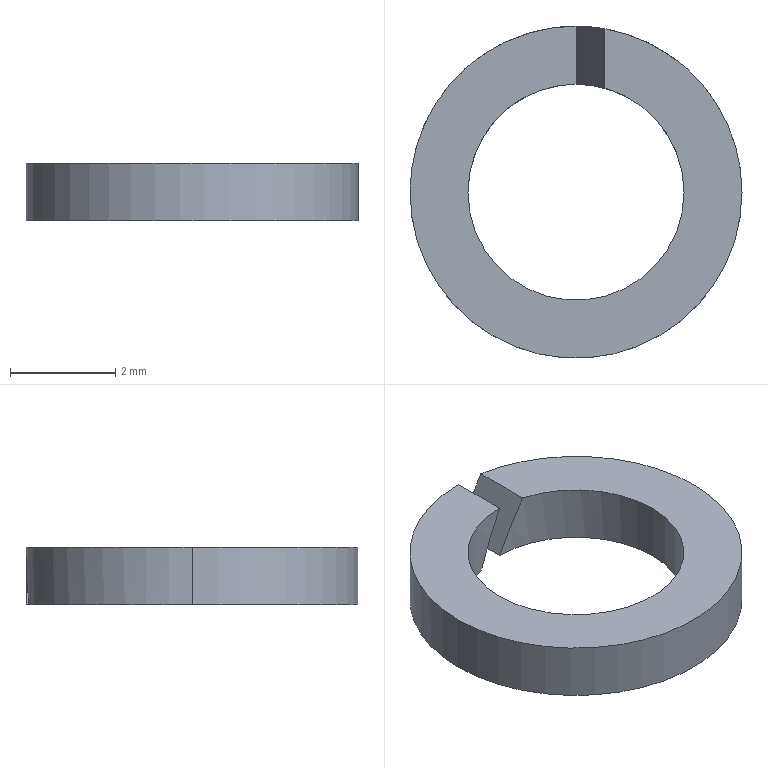Part | STEP file | Guide wheel mechanism revised.sldasm-Part-510 | 1 solid | 10 faces | box 6.3 x 6.3 x 1.1 mm | volume 19.099 mm3 | cylinder 6 | plane 4 | commonest cylinder face diameters 4.1 x3 6.3 x3
STEP:
#1=CARTESIAN_POINT('',(2.05,0.,0.));
#2=VERTEX_POINT('',#1);
#3=CARTESIAN_POINT('',(-2.05,0.,0.));
#4=VERTEX_POINT('',#3);
#5=CARTESIAN_POINT('',(0.,0.,0.));
#6=DIRECTION('',(0.,0.,-1.));
#7=DIRECTION('',(1.,0.,0.));
#8=AXIS2_PLACEMENT_3D('',#5,#6,#7);
#9=CIRCLE('',#8,2.05);
#10=EDGE_CURVE('',#2,#4,#9,.T.);
#11=ORIENTED_EDGE('',*,*,#10,.T.);
#12=CARTESIAN_POINT('',(-2.05,0.,1.1));
#13=VERTEX_POINT('',#12);
#14=CARTESIAN_POINT('',(-2.05,0.,0.));
#15=DIRECTION('',(0.,0.,1.));
#16=VECTOR('',#15,1000.);
#17=LINE('',#14,#16);
#18=EDGE_CURVE('',#4,#13,#17,.T.);
#19=ORIENTED_EDGE('',*,*,#18,.T.);
#20=CARTESIAN_POINT('',(2.05,0.,1.1));
#21=VERTEX_POINT('',#20);
#22=CARTESIAN_POINT('',(0.,0.,1.1));
#23=DIRECTION('',(0.,0.,-1.));
#24=DIRECTION('',(1.,0.,0.));
#25=AXIS2_PLACEMENT_3D('',#22,#23,#24);
#26=CIRCLE('',#25,2.05);
#27=EDGE_CURVE('',#21,#13,#26,.T.);
#28=ORIENTED_EDGE('',*,*,#27,.F.);
#29=CARTESIAN_POINT('',(2.05,0.,0.));
#30=DIRECTION('',(0.,0.,1.));
#31=VECTOR('',#30,1000.);
#32=LINE('',#29,#31);
#33=EDGE_CURVE('',#2,#21,#32,.T.);
#34=ORIENTED_EDGE('',*,*,#33,.F.);
#35=EDGE_LOOP('',(#11,#19,#28,#34));
#36=FACE_OUTER_BOUND('',#35,.T.);
#37=CARTESIAN_POINT('',(0.,0.,0.));
#38=DIRECTION('',(0.,0.,1.));
#39=DIRECTION('',(1.,0.,0.));
#40=AXIS2_PLACEMENT_3D('',#37,#38,#39);
#41=CYLINDRICAL_SURFACE('',#40,2.05);
#42=ADVANCED_FACE('',(#36),#41,.F.);
#43=CARTESIAN_POINT('',(0.,2.05,0.));
#44=VERTEX_POINT('',#43);
#45=CARTESIAN_POINT('',(0.,0.,0.));
#46=DIRECTION('',(0.,0.,-1.));
#47=DIRECTION('',(1.,0.,0.));
#48=AXIS2_PLACEMENT_3D('',#45,#46,#47);
#49=CIRCLE('',#48,2.05);
#50=EDGE_CURVE('',#44,#2,#49,.T.);
#51=ORIENTED_EDGE('',*,*,#50,.T.);
#52=ORIENTED_EDGE('',*,*,#33,.T.);
#53=CARTESIAN_POINT('',(0.55,1.975,1.1));
#54=VERTEX_POINT('',#53);
#55=CARTESIAN_POINT('',(0.,0.,1.1));
#56=DIRECTION('',(0.,0.,-1.));
#57=DIRECTION('',(1.,0.,0.));
#58=AXIS2_PLACEMENT_3D('',#55,#56,#57);
#59=CIRCLE('',#58,2.05);
#60=EDGE_CURVE('',#54,#21,#59,.T.);
#61=ORIENTED_EDGE('',*,*,#60,.F.);
#62=CARTESIAN_POINT('',(0.,2.05,0.));
#63=CARTESIAN_POINT('',(0.1862,2.05,0.3724));
#64=CARTESIAN_POINT('',(0.3706,2.025,0.7413));
#65=CARTESIAN_POINT('',(0.55,1.975,1.1));
#66=(BOUNDED_CURVE()B_SPLINE_CURVE(3,(#62,#63,#64,#65),.UNSPECIFIED.,.F.,.F.)B_SPLINE_CURVE_WITH_KNOTS((4,4),(4.712,4.984),.UNSPECIFIED.)CURVE()GEOMETRIC_REPRESENTATION_ITEM()RATIONAL_B_SPLINE_CURVE((1.,0.9939,0.9939,1.))REPRESENTATION_ITEM(''));
#67=EDGE_CURVE('',#44,#54,#66,.T.);
#68=ORIENTED_EDGE('',*,*,#67,.F.);
#69=EDGE_LOOP('',(#51,#52,#61,#68));
#70=FACE_OUTER_BOUND('',#69,.T.);
#71=CARTESIAN_POINT('',(0.,0.,0.));
#72=DIRECTION('',(0.,0.,1.));
#73=DIRECTION('',(1.,0.,0.));
#74=AXIS2_PLACEMENT_3D('',#71,#72,#73);
#75=CYLINDRICAL_SURFACE('',#74,2.05);
#76=ADVANCED_FACE('',(#70),#75,.F.);
#77=CARTESIAN_POINT('',(-0.55,3.102,0.));
#78=VERTEX_POINT('',#77);
#79=CARTESIAN_POINT('',(-3.15,0.,0.));
#80=VERTEX_POINT('',#79);
#81=CARTESIAN_POINT('',(0.,0.,0.));
#82=DIRECTION('',(0.,0.,1.));
#83=DIRECTION('',(1.,0.,0.));
#84=AXIS2_PLACEMENT_3D('',#81,#82,#83);
#85=CIRCLE('',#84,3.15);
#86=EDGE_CURVE('',#78,#80,#85,.T.);
#87=ORIENTED_EDGE('',*,*,#86,.T.);
#88=CARTESIAN_POINT('',(-3.15,0.,1.1));
#89=VERTEX_POINT('',#88);
#90=CARTESIAN_POINT('',(-3.15,0.,0.));
#91=DIRECTION('',(0.,0.,1.));
#92=VECTOR('',#91,1000.);
#93=LINE('',#90,#92);
#94=EDGE_CURVE('',#80,#89,#93,.T.);
#95=ORIENTED_EDGE('',*,*,#94,.T.);
#96=CARTESIAN_POINT('',(0.,3.15,1.1));
#97=VERTEX_POINT('',#96);
#98=CARTESIAN_POINT('',(0.,0.,1.1));
#99=DIRECTION('',(0.,0.,-1.));
#100=DIRECTION('',(1.,0.,0.));
#101=AXIS2_PLACEMENT_3D('',#98,#99,#100);
#102=CIRCLE('',#101,3.15);
#103=EDGE_CURVE('',#89,#97,#102,.T.);
#104=ORIENTED_EDGE('',*,*,#103,.T.);
#105=CARTESIAN_POINT('',(0.,3.15,1.1));
#106=CARTESIAN_POINT('',(-0.1845,3.15,0.731));
#107=CARTESIAN_POINT('',(-0.3683,3.134,0.3634));
#108=CARTESIAN_POINT('',(-0.55,3.102,0.));
#109=(BOUNDED_CURVE()B_SPLINE_CURVE(3,(#105,#106,#107,#108),.UNSPECIFIED.,.F.,.F.)B_SPLINE_CURVE_WITH_KNOTS((4,4),(1.571,1.746),.UNSPECIFIED.)CURVE()GEOMETRIC_REPRESENTATION_ITEM()RATIONAL_B_SPLINE_CURVE((1.,0.9974,0.9974,1.))REPRESENTATION_ITEM(''));
#110=EDGE_CURVE('',#97,#78,#109,.T.);
#111=ORIENTED_EDGE('',*,*,#110,.T.);
#112=EDGE_LOOP('',(#87,#95,#104,#111));
#113=FACE_OUTER_BOUND('',#112,.T.);
#114=CARTESIAN_POINT('',(0.,0.,0.));
#115=DIRECTION('',(0.,0.,1.));
#116=DIRECTION('',(1.,0.,0.));
#117=AXIS2_PLACEMENT_3D('',#114,#115,#116);
#118=CYLINDRICAL_SURFACE('',#117,3.15);
#119=ADVANCED_FACE('',(#113),#118,.T.);
#120=ORIENTED_EDGE('',*,*,#94,.F.);
#121=CARTESIAN_POINT('',(3.15,0.,0.));
#122=VERTEX_POINT('',#121);
#123=CARTESIAN_POINT('',(0.,0.,0.));
#124=DIRECTION('',(0.,0.,1.));
#125=DIRECTION('',(1.,0.,0.));
#126=AXIS2_PLACEMENT_3D('',#123,#124,#125);
#127=CIRCLE('',#126,3.15);
#128=EDGE_CURVE('',#80,#122,#127,.T.);
#129=ORIENTED_EDGE('',*,*,#128,.T.);
#130=CARTESIAN_POINT('',(3.15,0.,1.1));
#131=VERTEX_POINT('',#130);
#132=CARTESIAN_POINT('',(3.15,0.,0.));
#133=DIRECTION('',(0.,0.,1.));
#134=VECTOR('',#133,1000.);
#135=LINE('',#132,#134);
#136=EDGE_CURVE('',#122,#131,#135,.T.);
#137=ORIENTED_EDGE('',*,*,#136,.T.);
#138=CARTESIAN_POINT('',(0.,0.,1.1));
#139=DIRECTION('',(0.,0.,-1.));
#140=DIRECTION('',(1.,0.,0.));
#141=AXIS2_PLACEMENT_3D('',#138,#139,#140);
#142=CIRCLE('',#141,3.15);
#143=EDGE_CURVE('',#131,#89,#142,.T.);
#144=ORIENTED_EDGE('',*,*,#143,.T.);
#145=EDGE_LOOP('',(#120,#129,#137,#144));
#146=FACE_OUTER_BOUND('',#145,.T.);
#147=CARTESIAN_POINT('',(0.,0.,0.));
#148=DIRECTION('',(0.,0.,1.));
#149=DIRECTION('',(1.,0.,0.));
#150=AXIS2_PLACEMENT_3D('',#147,#148,#149);
#151=CYLINDRICAL_SURFACE('',#150,3.15);
#152=ADVANCED_FACE('',(#146),#151,.T.);
#153=ORIENTED_EDGE('',*,*,#50,.F.);
#154=CARTESIAN_POINT('',(0.,3.15,0.));
#155=VERTEX_POINT('',#154);
#156=CARTESIAN_POINT('',(0.,0.,0.));
#157=DIRECTION('',(0.,-1.,0.));
#158=VECTOR('',#157,1000.);
#159=LINE('',#156,#158);
#160=EDGE_CURVE('',#155,#44,#159,.T.);
#161=ORIENTED_EDGE('',*,*,#160,.F.);
#162=CARTESIAN_POINT('',(0.,0.,0.));
#163=DIRECTION('',(0.,0.,1.));
#164=DIRECTION('',(1.,0.,0.));
#165=AXIS2_PLACEMENT_3D('',#162,#163,#164);
#166=CIRCLE('',#165,3.15);
#167=EDGE_CURVE('',#122,#155,#166,.T.);
#168=ORIENTED_EDGE('',*,*,#167,.F.);
#169=ORIENTED_EDGE('',*,*,#128,.F.);
#170=ORIENTED_EDGE('',*,*,#86,.F.);
#171=CARTESIAN_POINT('',(-0.55,1.975,0.));
#172=VERTEX_POINT('',#171);
#173=CARTESIAN_POINT('',(-0.55,0.,0.));
#174=DIRECTION('',(0.,1.,0.));
#175=VECTOR('',#174,1000.);
#176=LINE('',#173,#175);
#177=EDGE_CURVE('',#172,#78,#176,.T.);
#178=ORIENTED_EDGE('',*,*,#177,.F.);
#179=CARTESIAN_POINT('',(0.,0.,0.));
#180=DIRECTION('',(0.,0.,-1.));
#181=DIRECTION('',(1.,0.,0.));
#182=AXIS2_PLACEMENT_3D('',#179,#180,#181);
#183=CIRCLE('',#182,2.05);
#184=EDGE_CURVE('',#4,#172,#183,.T.);
#185=ORIENTED_EDGE('',*,*,#184,.F.);
#186=ORIENTED_EDGE('',*,*,#10,.F.);
#187=EDGE_LOOP('',(#153,#161,#168,#169,#170,#178,#185,#186));
#188=FACE_OUTER_BOUND('',#187,.T.);
#189=CARTESIAN_POINT('',(0.,0.,0.));
#190=DIRECTION('',(0.,0.,1.));
#191=DIRECTION('',(1.,0.,0.));
#192=AXIS2_PLACEMENT_3D('',#189,#190,#191);
#193=PLANE('',#192);
#194=ADVANCED_FACE('',(#188),#193,.F.);
#195=ORIENTED_EDGE('',*,*,#18,.F.);
#196=ORIENTED_EDGE('',*,*,#184,.T.);
#197=CARTESIAN_POINT('',(0.,2.05,1.1));
#198=VERTEX_POINT('',#197);
#199=CARTESIAN_POINT('',(0.,2.05,1.1));
#200=CARTESIAN_POINT('',(-0.1862,2.05,0.7276));
#201=CARTESIAN_POINT('',(-0.3706,2.025,0.3587));
#202=CARTESIAN_POINT('',(-0.55,1.975,0.));
#203=(BOUNDED_CURVE()B_SPLINE_CURVE(3,(#199,#200,#201,#202),.UNSPECIFIED.,.F.,.F.)B_SPLINE_CURVE_WITH_KNOTS((4,4),(1.571,1.842),.UNSPECIFIED.)CURVE()GEOMETRIC_REPRESENTATION_ITEM()RATIONAL_B_SPLINE_CURVE((1.,0.9939,0.9939,1.))REPRESENTATION_ITEM(''));
#204=EDGE_CURVE('',#198,#172,#203,.T.);
#205=ORIENTED_EDGE('',*,*,#204,.F.);
#206=CARTESIAN_POINT('',(0.,0.,1.1));
#207=DIRECTION('',(0.,0.,-1.));
#208=DIRECTION('',(1.,0.,0.));
#209=AXIS2_PLACEMENT_3D('',#206,#207,#208);
#210=CIRCLE('',#209,2.05);
#211=EDGE_CURVE('',#13,#198,#210,.T.);
#212=ORIENTED_EDGE('',*,*,#211,.F.);
#213=EDGE_LOOP('',(#195,#196,#205,#212));
#214=FACE_OUTER_BOUND('',#213,.T.);
#215=CARTESIAN_POINT('',(0.,0.,0.));
#216=DIRECTION('',(0.,0.,1.));
#217=DIRECTION('',(1.,0.,0.));
#218=AXIS2_PLACEMENT_3D('',#215,#216,#217);
#219=CYLINDRICAL_SURFACE('',#218,2.05);
#220=ADVANCED_FACE('',(#214),#219,.F.);
#221=ORIENTED_EDGE('',*,*,#67,.T.);
#222=CARTESIAN_POINT('',(0.55,3.102,1.1));
#223=VERTEX_POINT('',#222);
#224=CARTESIAN_POINT('',(0.55,0.,1.1));
#225=DIRECTION('',(0.,-1.,0.));
#226=VECTOR('',#225,1000.);
#227=LINE('',#224,#226);
#228=EDGE_CURVE('',#223,#54,#227,.T.);
#229=ORIENTED_EDGE('',*,*,#228,.F.);
#230=CARTESIAN_POINT('',(0.,3.15,0.));
#231=CARTESIAN_POINT('',(0.1845,3.15,0.369));
#232=CARTESIAN_POINT('',(0.3683,3.134,0.7366));
#233=CARTESIAN_POINT('',(0.55,3.102,1.1));
#234=(BOUNDED_CURVE()B_SPLINE_CURVE(3,(#230,#231,#232,#233),.UNSPECIFIED.,.F.,.F.)B_SPLINE_CURVE_WITH_KNOTS((4,4),(4.712,4.888),.UNSPECIFIED.)CURVE()GEOMETRIC_REPRESENTATION_ITEM()RATIONAL_B_SPLINE_CURVE((1.,0.9974,0.9974,1.))REPRESENTATION_ITEM(''));
#235=EDGE_CURVE('',#155,#223,#234,.T.);
#236=ORIENTED_EDGE('',*,*,#235,.F.);
#237=ORIENTED_EDGE('',*,*,#160,.T.);
#238=EDGE_LOOP('',(#221,#229,#236,#237));
#239=FACE_OUTER_BOUND('',#238,.T.);
#240=CARTESIAN_POINT('',(0.55,0.,1.1));
#241=DIRECTION('',(0.8944,0.,-0.4472));
#242=DIRECTION('',(-0.4472,0.,-0.8944));
#243=AXIS2_PLACEMENT_3D('',#240,#241,#242);
#244=PLANE('',#243);
#245=ADVANCED_FACE('',(#239),#244,.F.);
#246=ORIENTED_EDGE('',*,*,#136,.F.);
#247=ORIENTED_EDGE('',*,*,#167,.T.);
#248=ORIENTED_EDGE('',*,*,#235,.T.);
#249=CARTESIAN_POINT('',(0.,0.,1.1));
#250=DIRECTION('',(0.,0.,-1.));
#251=DIRECTION('',(1.,0.,0.));
#252=AXIS2_PLACEMENT_3D('',#249,#250,#251);
#253=CIRCLE('',#252,3.15);
#254=EDGE_CURVE('',#223,#131,#253,.T.);
#255=ORIENTED_EDGE('',*,*,#254,.T.);
#256=EDGE_LOOP('',(#246,#247,#248,#255));
#257=FACE_OUTER_BOUND('',#256,.T.);
#258=CARTESIAN_POINT('',(0.,0.,0.));
#259=DIRECTION('',(0.,0.,1.));
#260=DIRECTION('',(1.,0.,0.));
#261=AXIS2_PLACEMENT_3D('',#258,#259,#260);
#262=CYLINDRICAL_SURFACE('',#261,3.15);
#263=ADVANCED_FACE('',(#257),#262,.T.);
#264=ORIENTED_EDGE('',*,*,#110,.F.);
#265=CARTESIAN_POINT('',(0.,0.,1.1));
#266=DIRECTION('',(0.,1.,0.));
#267=VECTOR('',#266,1000.);
#268=LINE('',#265,#267);
#269=EDGE_CURVE('',#198,#97,#268,.T.);
#270=ORIENTED_EDGE('',*,*,#269,.F.);
#271=ORIENTED_EDGE('',*,*,#204,.T.);
#272=ORIENTED_EDGE('',*,*,#177,.T.);
#273=EDGE_LOOP('',(#264,#270,#271,#272));
#274=FACE_OUTER_BOUND('',#273,.T.);
#275=CARTESIAN_POINT('',(-0.55,0.,0.));
#276=DIRECTION('',(-0.8944,0.,0.4472));
#277=DIRECTION('',(0.4472,0.,0.8944));
#278=AXIS2_PLACEMENT_3D('',#275,#276,#277);
#279=PLANE('',#278);
#280=ADVANCED_FACE('',(#274),#279,.F.);
#281=ORIENTED_EDGE('',*,*,#60,.T.);
#282=ORIENTED_EDGE('',*,*,#27,.T.);
#283=ORIENTED_EDGE('',*,*,#211,.T.);
#284=ORIENTED_EDGE('',*,*,#269,.T.);
#285=ORIENTED_EDGE('',*,*,#103,.F.);
#286=ORIENTED_EDGE('',*,*,#143,.F.);
#287=ORIENTED_EDGE('',*,*,#254,.F.);
#288=ORIENTED_EDGE('',*,*,#228,.T.);
#289=EDGE_LOOP('',(#281,#282,#283,#284,#285,#286,#287,#288));
#290=FACE_OUTER_BOUND('',#289,.T.);
#291=CARTESIAN_POINT('',(0.,0.,1.1));
#292=DIRECTION('',(0.,0.,1.));
#293=DIRECTION('',(1.,0.,0.));
#294=AXIS2_PLACEMENT_3D('',#291,#292,#293);
#295=PLANE('',#294);
#296=ADVANCED_FACE('',(#290),#295,.T.);
#297=CLOSED_SHELL('',(#42,#76,#119,#152,#194,#220,#245,#263,#280,#296));
#298=MANIFOLD_SOLID_BREP('',#297);
#299=CARTESIAN_POINT('',(0.,0.,0.));
#300=DIRECTION('',(0.,0.,1.));
#301=DIRECTION('',(1.,0.,0.));
#302=AXIS2_PLACEMENT_3D('',#299,#300,#301);
#303=(LENGTH_UNIT()NAMED_UNIT(*)SI_UNIT(.MILLI.,.METRE.));
#304=UNCERTAINTY_MEASURE_WITH_UNIT(LENGTH_MEASURE(0.00001),#303,'','');
#305=(NAMED_UNIT(*)PLANE_ANGLE_UNIT()SI_UNIT($,.RADIAN.));
#306=(NAMED_UNIT(*)SI_UNIT($,.STERADIAN.)SOLID_ANGLE_UNIT());
#307=(GEOMETRIC_REPRESENTATION_CONTEXT(3)GLOBAL_UNCERTAINTY_ASSIGNED_CONTEXT((#304))GLOBAL_UNIT_ASSIGNED_CONTEXT((#303,#305,#306))REPRESENTATION_CONTEXT('',''));
#308=ADVANCED_BREP_SHAPE_REPRESENTATION('',(#298,#302),#307);